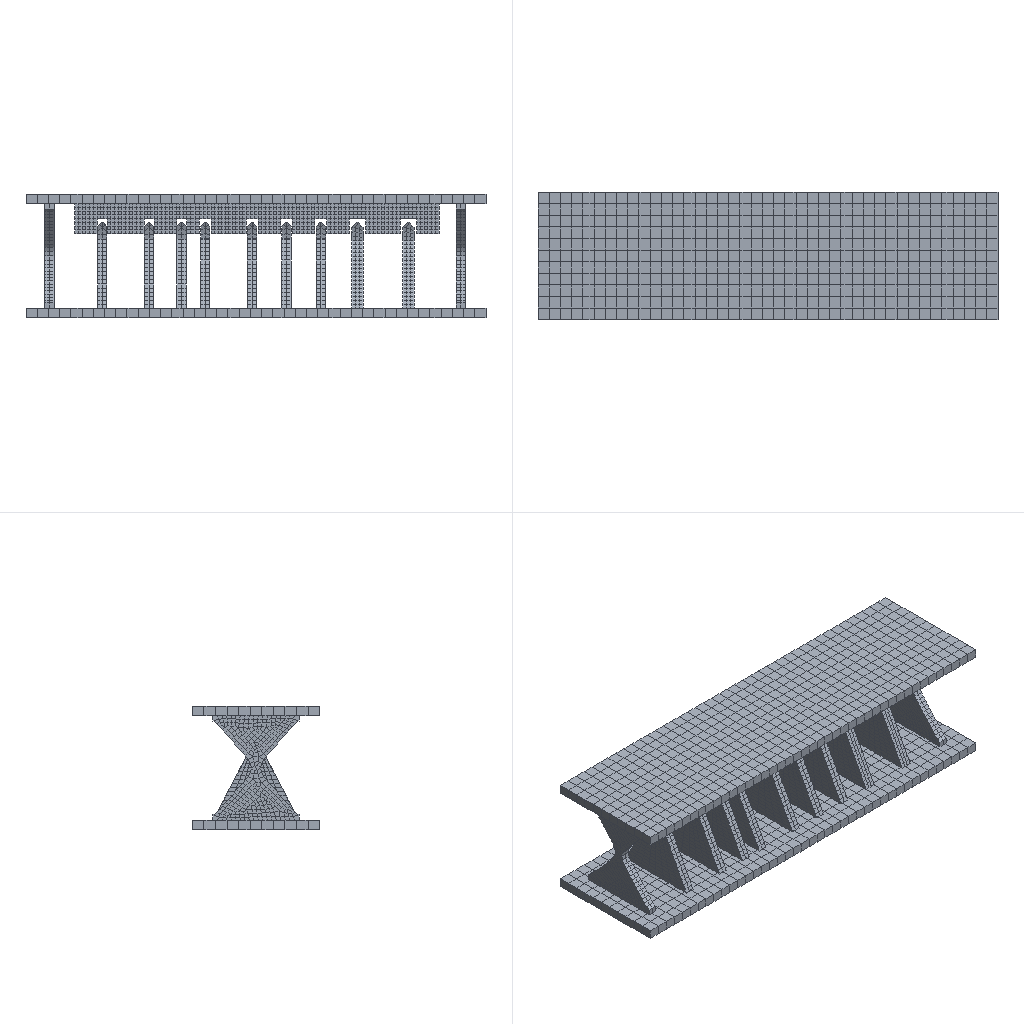Simulation study | abaqus
Abaqus input file, long lists of numbers shortened:
*Heading
** Job name: deck-1 Model name: 0814
** Generated by: Abaqus/CAE 2024
*Preprint, echo=NO, model=NO, history=NO, contact=NO
**
** PARTS
**
*Part, name=Part-1
*Node
      1,      1227.62,         340.,          25.
      2,      1227.62,   309.091,          25.
** (1006 more lines like these left out)
*Element, type=C3D8R
  1,   25,   26,   38,   37,    1,    2,   14,   13
  2,   26,   27,   39,   38,    2,    3,   15,   14
** (449 more lines like these left out)
*Nset, nset=_PickedSet5, internal, generate
    1,  1008,     1
*Elset, elset=_PickedSet5, internal, generate
   1,  451,    1
** Section: q235
*Solid Section, elset=_PickedSet5, controls=EC-1, material=q235
,
*End Part
**
*Part, name=Part-7
*Node
      1,   51318.848,   20056.129,           0.
      2,      51308.5,   20050.193,           0.
** (1084 more lines like these left out)
*Element, type=C3D8R
  1,  119,    1,    2,  145,  481,  363,  364,  507
  2,    1,  119,  116,   23,  363,  481,  478,  385
** (622 more lines like these left out)
*Nset, nset=Set-1, generate
    1,  1086,     1
*Elset, elset=Set-1, generate
   1,  624,    1
** Section: Section-2
*Solid Section, elset=Set-1, material=q235
,
*End Part
**
*Part, name=Part-8
*Node
      1,   44.972,         218.,           0.
      2,   50.449,         230.,          10.
** (601 more lines like these left out)
*Element, type=C3D8R
 1, 164,  20, 157, 481,  18,   1,  19, 155
 2, 165,  21, 158, 480, 164,  20, 157, 481
** (334 more lines like these left out)
*Nset, nset=Set-1, generate
   1,  603,    1
*Elset, elset=Set-1, generate
   1,  336,    1
** Section: Section-2
*Solid Section, elset=Set-1, material=q235
,
*End Part
**
*Part, name=Part-9
*Node
      1,  -916.483,   84.154,           0.
      2,  -916.483,   84.154,          40.
** (4008 more lines like these left out)
*Element, type=C3D8R
 1,  158, 1029, 2787,  999,    1,  121,  969,  136
 2, 1029, 1030, 2788, 2787,  121,  122,  970,  969
** (2638 more lines like these left out)
*Nset, nset=Set-1, generate
    1,  4010,     1
*Elset, elset=Set-1, generate
    1,  2640,     1
** Section: Section-2
*Solid Section, elset=Set-1, material=q235
,
*End Part
**
*Part, name=Part-10
*Node
      1,   4.129,   256.243,          25.
      2,   4.785,   252.357,          25.
** (558 more lines like these left out)
*Element, type=C3D8R
 1,  36,  43, 171, 165,   1,   2,  21,  22
 2, 165, 171,  42,  25,  22,  21,   3,   4
** (306 more lines like these left out)
*Nset, nset=Set-1
   1,   2,   3,   4,   5,   6,   7,   8,  17,  18,  19,  20,  21,  22,  23,  24
  25,  26,  27,  28,  29,  30,  31,  32,  33,  34,  35,  36,  37,  38,  39,  40
** (27 more lines like these left out)
*Elset, elset=Set-1
   1,   2,   3,   4,   5,   6,   7,   8,   9,  10,  11,  12,  13,  14,  71,  72
  73,  74,  75,  76,  77,  78,  79,  80,  81,  82,  83,  84,  85,  86,  87,  88
** (14 more lines like these left out)
*Nset, nset=_PickedSet10, internal, generate
   1,  560,    1
*Elset, elset=_PickedSet10, internal, generate
   1,  308,    1
** Section: Section-2
*Solid Section, elset=_PickedSet10, material=q235
,
*End Part
**
*Part, name=Part-11
*Node
      1,  -175.665,   409.503,         17.5
      2,  -105.665,   409.503,         17.5
** (878 more lines like these left out)
*Element, type=C3D8R
  1,   4,  22,   7,   1,  44,  62,  47,  41
  2,  22,  21,   8,   7,  62,  61,  48,  47
** (565 more lines like these left out)
*Nset, nset=Set-1, generate
   1,  880,    1
*Elset, elset=Set-1, generate
   1,  567,    1
** Section: Section-2
*Solid Section, elset=Set-1, material=q235
,
*End Part
**
**
** ASSEMBLY
**
*Assembly, name=Assembly
**
*Instance, name=Part-1-1, part=Part-1
*End Instance
**
*Instance, name=Part-1-1-lin-2-1, part=Part-1
          0.,           0.,         305.
*End Instance
**
*Instance, name=Part-7-1, part=Part-7
50.,     -51253.5, -20010.046
50.,     -51253.5, -20010.046, 50.577, -51252.923, -20009.469,         120.
*End Instance
**
*Instance, name=Part-7-1-lin-2-1, part=Part-7
     1147.62,     -51253.5, -20010.046
     1147.62,     -51253.5, -20010.046, 1148.197, -51252.923, -20009.469,         120.
*End Instance
**
*Instance, name=Part-9-1, part=Part-9
 1106.483,         190.,   180.846
 1106.483,         190.,   180.846, 1107.483,         190.,   180.846, 90.
*End Instance
**
*Instance, name=Part-8-1, part=Part-8
      190.85,   152.051,          25.
      190.85,   152.051,          25., 191.427, 152.628, 25.577,         120.
*End Instance
**
*Instance, name=Part-8-1-lin-1-2, part=Part-8
      315.85,   152.051,          25.
      315.85,   152.051,          25., 316.427, 152.628, 25.577,         120.
*End Instance
**
*Instance, name=Part-8-1-lin-1-2-lin-2-1, part=Part-8
      402.55,   152.051,          25.
      402.55,   152.051,          25., 403.127, 152.628, 25.577,         120.
*End Instance
**
*Instance, name=Part-10-1, part=Part-10
      465.85,   184.157,    -44.124
      465.85,   184.157,    -44.124, 466.427, 184.734, -43.547,         120.
*End Instance
**
*Instance, name=Part-10-1-lin-2-1, part=Part-10
      590.85,   184.157,    -44.124
      590.85,   184.157,    -44.124, 591.427, 184.734, -43.547,         120.
*End Instance
**
*Instance, name=Part-10-1-lin-3-1, part=Part-10
      774.37,   184.157,    -44.124
      774.37,   184.157,    -44.124, 774.947, 184.734, -43.547,         120.
*End Instance
**
*Instance, name=Part-10-1-lin-4-1, part=Part-10
      682.61,   184.157,    -44.124
      682.61,   184.157,    -44.124, 683.187, 184.734, -43.547,         120.
*End Instance
**
*Instance, name=Part-11-1, part=Part-11
      869.52,   310.665,   -154.503
      869.52,   310.665,   -154.503, 870.097, 311.242, -153.925,         120.
*End Instance
**
*Instance, name=Part-11-1-lin-2-1, part=Part-11
     1005.85,   310.665,   -154.503
     1005.85,   310.665,   -154.503, 1006.427, 311.242, -153.925,         120.
*End Instance
**
*Node
      1,   613.81,         170.,         500.
*Node
      2,   613.81,         170.,        -200.
*Nset, nset=Set-1, instance=Part-1-1
   13,   14,   15,   16,   17,   18,   19,   20,   21,   22,   23,   24,   37,   38,   39,   40
   41,   42,   43,   44,   45,   46,   47,   48,   61,   62,   63,   64,   65,   66,   67,   68
** (30 more lines like these left out)
*Elset, elset=Set-1, instance=Part-1-1, generate
   1,  451,    1
*Nset, nset=Set-6
 2,
*Nset, nset=Set-7
 1,
*Nset, nset=m_Set-5
 2,
*Nset, nset=rp1
 1,
*Nset, nset=rp2
 2,
*Nset, nset=_PickedSet71, internal
 1,
*Nset, nset=_PickedSet120, internal
 1,
*Nset, nset=_PickedSet121, internal
 2,
*Elset, elset=_m_Surf-12_S5, internal, instance=Part-1-1-lin-2-1, generate
   1,  451,    1
*Surface, type=ELEMENT, name=m_Surf-12
_m_Surf-12_S5, S5
*Elset, elset=_m_Surf-13_S3, internal, instance=Part-1-1, generate
   1,  451,    1
*Surface, type=ELEMENT, name=m_Surf-13
_m_Surf-13_S3, S3
*Elset, elset=_m_Surf-17_S3, internal, instance=Part-1-1, generate
   1,  451,    1
*Surface, type=ELEMENT, name=m_Surf-17
_m_Surf-17_S3, S3
*Elset, elset=_m_Surf-19_S5, internal, instance=Part-1-1-lin-2-1, generate
   1,  451,    1
*Surface, type=ELEMENT, name=m_Surf-19
_m_Surf-19_S5, S5
*Elset, elset=_m_Surf-28_S5, internal, instance=Part-8-1
  82,  83,  84,  85,  86,  87,  88,  89,  90,  91,  92,  93,  94,  95,  96,  97
  98, 116, 117, 118, 119, 120, 121, 122, 123, 124, 125, 126, 127, 128, 129, 130
** (7 more lines like these left out)
*Elset, elset=_m_Surf-28_S5, internal, instance=Part-8-1-lin-1-2
  82,  83,  84,  85,  86,  87,  88,  89,  90,  91,  92,  93,  94,  95,  96,  97
  98, 116, 117, 118, 119, 120, 121, 122, 123, 124, 125, 126, 127, 128, 129, 130
** (7 more lines like these left out)
*Elset, elset=_m_Surf-28_S5, internal, instance=Part-8-1-lin-1-2-lin-2-1
  82,  83,  84,  85,  86,  87,  88,  89,  90,  91,  92,  93,  94,  95,  96,  97
  98, 116, 117, 118, 119, 120, 121, 122, 123, 124, 125, 126, 127, 128, 129, 130
** (7 more lines like these left out)
*Elset, elset=_m_Surf-28_S5, internal, instance=Part-10-1-lin-2-1, generate
  2,  14,   2
*Elset, elset=_m_Surf-28_S5, internal, instance=Part-10-1-lin-4-1, generate
  2,  14,   2
*Elset, elset=_m_Surf-28_S5, internal, instance=Part-10-1, generate
  2,  14,   2
*Elset, elset=_m_Surf-28_S5, internal, instance=Part-10-1-lin-3-1, generate
  2,  14,   2
*Elset, elset=_m_Surf-28_S3, internal, instance=Part-8-1
  65,  66,  67,  68,  69,  70,  71,  72,  73,  74,  75,  76,  77,  78,  79,  80
  81,  99, 100, 101, 102, 103, 104, 105, 106, 107, 108, 109, 110, 111, 112, 113
** (7 more lines like these left out)
*Elset, elset=_m_Surf-28_S3, internal, instance=Part-8-1-lin-1-2
  65,  66,  67,  68,  69,  70,  71,  72,  73,  74,  75,  76,  77,  78,  79,  80
  81,  99, 100, 101, 102, 103, 104, 105, 106, 107, 108, 109, 110, 111, 112, 113
** (7 more lines like these left out)
*Elset, elset=_m_Surf-28_S3, internal, instance=Part-8-1-lin-1-2-lin-2-1
  65,  66,  67,  68,  69,  70,  71,  72,  73,  74,  75,  76,  77,  78,  79,  80
  81,  99, 100, 101, 102, 103, 104, 105, 106, 107, 108, 109, 110, 111, 112, 113
** (7 more lines like these left out)
*Elset, elset=_m_Surf-28_S3, internal, instance=Part-10-1-lin-2-1, generate
  1,  13,   2
*Elset, elset=_m_Surf-28_S3, internal, instance=Part-10-1-lin-4-1, generate
  1,  13,   2
*Elset, elset=_m_Surf-28_S3, internal, instance=Part-10-1, generate
  1,  13,   2
*Elset, elset=_m_Surf-28_S3, internal, instance=Part-10-1-lin-3-1, generate
  1,  13,   2
*Elset, elset=_m_Surf-28_S4, internal, instance=Part-10-1-lin-2-1, generate
  72,  308,    2
*Elset, elset=_m_Surf-28_S4, internal, instance=Part-10-1-lin-4-1, generate
  72,  308,    2
*Elset, elset=_m_Surf-28_S4, internal, instance=Part-10-1, generate
  72,  308,    2
*Elset, elset=_m_Surf-28_S4, internal, instance=Part-10-1-lin-3-1, generate
  72,  308,    2
*Elset, elset=_m_Surf-28_S6, internal, instance=Part-10-1-lin-2-1, generate
  71,  307,    2
*Elset, elset=_m_Surf-28_S6, internal, instance=Part-10-1-lin-4-1, generate
  71,  307,    2
*Elset, elset=_m_Surf-28_S6, internal, instance=Part-10-1, generate
  71,  307,    2
*Elset, elset=_m_Surf-28_S6, internal, instance=Part-10-1-lin-3-1, generate
  71,  307,    2
*Elset, elset=_m_Surf-28_S1, internal, instance=Part-10-1-lin-2-1
 13, 14
*Elset, elset=_m_Surf-28_S1, internal, instance=Part-10-1-lin-4-1
 13, 14
*Elset, elset=_m_Surf-28_S1, internal, instance=Part-10-1
 13, 14
*Elset, elset=_m_Surf-28_S1, internal, instance=Part-10-1-lin-3-1
 13, 14
*Elset, elset=_m_Surf-28_S2, internal, instance=Part-10-1-lin-2-1
 1, 2
*Elset, elset=_m_Surf-28_S2, internal, instance=Part-10-1-lin-4-1
 1, 2
*Elset, elset=_m_Surf-28_S2, internal, instance=Part-10-1
 1, 2
*Elset, elset=_m_Surf-28_S2, internal, instance=Part-10-1-lin-3-1
 1, 2
*Surface, type=ELEMENT, name=m_Surf-28
_m_Surf-28_S5, S5
_m_Surf-28_S3, S3
_m_Surf-28_S4, S4
_m_Surf-28_S6, S6
_m_Surf-28_S2, S2
_m_Surf-28_S1, S1
*Elset, elset=_m_Surf-30_S4, internal, instance=Part-8-1
  1,  2,  3,  4,  5,  6,  7,  8,  9, 10, 11, 12, 13, 14, 15, 16
 25, 26, 27, 28, 29, 30, 31, 32, 36, 37, 38, 39, 40, 44, 48, 52
** (1 more lines like these left out)
*Elset, elset=_m_Surf-30_S4, internal, instance=Part-8-1-lin-1-2
  1,  2,  3,  4,  5,  6,  7,  8,  9, 10, 11, 12, 13, 14, 15, 16
 25, 26, 27, 28, 29, 30, 31, 32, 36, 37, 38, 39, 40, 44, 48, 52
** (1 more lines like these left out)
*Elset, elset=_m_Surf-30_S4, internal, instance=Part-8-1-lin-1-2-lin-2-1
  1,  2,  3,  4,  5,  6,  7,  8,  9, 10, 11, 12, 13, 14, 15, 16
 25, 26, 27, 28, 29, 30, 31, 32, 36, 37, 38, 39, 40, 44, 48, 52
** (1 more lines like these left out)
*Elset, elset=_m_Surf-30_S4, internal, instance=Part-10-1-lin-2-1
  15,  16,  17,  18,  19,  20,  21,  22,  23,  24,  25,  26,  33,  34,  35,  36
  37,  38,  42,  43,  44,  45,  46,  50,  54,  58,  62,  66,  70,  72,  74,  76
** (8 more lines like these left out)
*Elset, elset=_m_Surf-30_S4, internal, instance=Part-10-1-lin-4-1
  15,  16,  17,  18,  19,  20,  21,  22,  23,  24,  25,  26,  33,  34,  35,  36
  37,  38,  42,  43,  44,  45,  46,  50,  54,  58,  62,  66,  70,  72,  74,  76
** (8 more lines like these left out)
*Elset, elset=_m_Surf-30_S4, internal, instance=Part-11-1-lin-2-1, generate
   9,  549,   27
*Elset, elset=_m_Surf-30_S4, internal, instance=Part-10-1
  15,  16,  17,  18,  19,  20,  21,  22,  23,  24,  25,  26,  33,  34,  35,  36
  37,  38,  42,  43,  44,  45,  46,  50,  54,  58,  62,  66,  70,  72,  74,  76
** (8 more lines like these left out)
*Elset, elset=_m_Surf-30_S4, internal, instance=Part-11-1, generate
   9,  549,   27
*Elset, elset=_m_Surf-30_S4, internal, instance=Part-10-1-lin-3-1
  15,  16,  17,  18,  19,  20,  21,  22,  23,  24,  25,  26,  33,  34,  35,  36
  37,  38,  42,  43,  44,  45,  46,  50,  54,  58,  62,  66,  70,  72,  74,  76
** (8 more lines like these left out)
*Elset, elset=_m_Surf-30_S3, internal, instance=Part-8-1
   1,   2,   3,   4,   5,   6,   7,   8,   9,  10,  11,  12,  13,  14,  15,  16
  17,  18,  19,  20,  21,  22,  23,  24,  33,  34,  35,  36,  37,  49,  50,  51
** (10 more lines like these left out)
*Elset, elset=_m_Surf-30_S3, internal, instance=Part-8-1-lin-1-2
   1,   2,   3,   4,   5,   6,   7,   8,   9,  10,  11,  12,  13,  14,  15,  16
  17,  18,  19,  20,  21,  22,  23,  24,  33,  34,  35,  36,  37,  49,  50,  51
** (10 more lines like these left out)
*Elset, elset=_m_Surf-30_S3, internal, instance=Part-8-1-lin-1-2-lin-2-1
   1,   2,   3,   4,   5,   6,   7,   8,   9,  10,  11,  12,  13,  14,  15,  16
  17,  18,  19,  20,  21,  22,  23,  24,  33,  34,  35,  36,  37,  49,  50,  51
** (10 more lines like these left out)
*Elset, elset=_m_Surf-30_S3, internal, instance=Part-10-1-lin-2-1
   1,   3,   5,   7,   9,  11,  13,  15,  16,  17,  18,  19,  20,  21,  22,  23
  24,  25,  26,  27,  28,  29,  30,  31,  32,  39,  40,  41,  42,  43,  55,  56
** (3 more lines like these left out)
*Elset, elset=_m_Surf-30_S3, internal, instance=Part-10-1-lin-4-1
   1,   3,   5,   7,   9,  11,  13,  15,  16,  17,  18,  19,  20,  21,  22,  23
  24,  25,  26,  27,  28,  29,  30,  31,  32,  39,  40,  41,  42,  43,  55,  56
** (3 more lines like these left out)
*Elset, elset=_m_Surf-30_S3, internal, instance=Part-11-1-lin-2-1
   1,   2,   3,   4,   5,   6,   7,   8,   9,  26,  27,  28,  29,  30,  31,  32
  33,  34,  35,  36,  53,  54,  55,  56,  57,  58,  59,  60,  61,  62,  63,  80
** (13 more lines like these left out)
*Elset, elset=_m_Surf-30_S3, internal, instance=Part-10-1
   1,   3,   5,   7,   9,  11,  13,  15,  16,  17,  18,  19,  20,  21,  22,  23
  24,  25,  26,  27,  28,  29,  30,  31,  32,  39,  40,  41,  42,  43,  55,  56
** (3 more lines like these left out)
*Elset, elset=_m_Surf-30_S3, internal, instance=Part-11-1
   1,   2,   3,   4,   5,   6,   7,   8,   9,  26,  27,  28,  29,  30,  31,  32
  33,  34,  35,  36,  53,  54,  55,  56,  57,  58,  59,  60,  61,  62,  63,  80
** (13 more lines like these left out)
*Elset, elset=_m_Surf-30_S3, internal, instance=Part-10-1-lin-3-1
   1,   3,   5,   7,   9,  11,  13,  15,  16,  17,  18,  19,  20,  21,  22,  23
  24,  25,  26,  27,  28,  29,  30,  31,  32,  39,  40,  41,  42,  43,  55,  56
** (3 more lines like these left out)
*Elset, elset=_m_Surf-30_S2, internal, instance=Part-8-1
  1,  5,  9, 13, 17, 18, 25, 26, 33, 34, 35, 36, 37, 38, 39, 40
 41, 42, 43, 44, 45, 46, 47, 48, 57, 61, 65, 66, 67, 68, 69, 70
** (2 more lines like these left out)
*Elset, elset=_m_Surf-30_S2, internal, instance=Part-8-1-lin-1-2
  1,  5,  9, 13, 17, 18, 25, 26, 33, 34, 35, 36, 37, 38, 39, 40
 41, 42, 43, 44, 45, 46, 47, 48, 57, 61, 65, 66, 67, 68, 69, 70
** (2 more lines like these left out)
*Elset, elset=_m_Surf-30_S2, internal, instance=Part-8-1-lin-1-2-lin-2-1
  1,  5,  9, 13, 17, 18, 25, 26, 33, 34, 35, 36, 37, 38, 39, 40
 41, 42, 43, 44, 45, 46, 47, 48, 57, 61, 65, 66, 67, 68, 69, 70
** (2 more lines like these left out)
*Elset, elset=_m_Surf-30_S2, internal, instance=Part-10-1-lin-2-1
  1,  2, 15, 18, 21, 24, 27, 28, 33, 34, 39, 40, 41, 42, 43, 44
 45, 46, 47, 48, 49, 50, 51, 52, 53, 54, 63, 64, 65, 66, 67, 68
** (1 more lines like these left out)
*Elset, elset=_m_Surf-30_S2, internal, instance=Part-10-1-lin-4-1
  1,  2, 15, 18, 21, 24, 27, 28, 33, 34, 39, 40, 41, 42, 43, 44
 45, 46, 47, 48, 49, 50, 51, 52, 53, 54, 63, 64, 65, 66, 67, 68
** (1 more lines like these left out)
*Elset, elset=_m_Surf-30_S2, internal, instance=Part-10-1
  1,  2, 15, 18, 21, 24, 27, 28, 33, 34, 39, 40, 41, 42, 43, 44
 45, 46, 47, 48, 49, 50, 51, 52, 53, 54, 63, 64, 65, 66, 67, 68
** (1 more lines like these left out)
*Elset, elset=_m_Surf-30_S2, internal, instance=Part-10-1-lin-3-1
  1,  2, 15, 18, 21, 24, 27, 28, 33, 34, 39, 40, 41, 42, 43, 44
 45, 46, 47, 48, 49, 50, 51, 52, 53, 54, 63, 64, 65, 66, 67, 68
** (1 more lines like these left out)
*Elset, elset=_m_Surf-30_S5, internal, instance=Part-8-1
  82,  83,  84,  85,  86,  87,  88,  89,  90,  91,  92,  93,  94,  95,  96,  97
  98, 116, 117, 118, 119, 120, 121, 122, 123, 124, 125, 126, 127, 128, 129, 130
** (7 more lines like these left out)
*Elset, elset=_m_Surf-30_S5, internal, instance=Part-8-1-lin-1-2
  82,  83,  84,  85,  86,  87,  88,  89,  90,  91,  92,  93,  94,  95,  96,  97
  98, 116, 117, 118, 119, 120, 121, 122, 123, 124, 125, 126, 127, 128, 129, 130
** (7 more lines like these left out)
*Elset, elset=_m_Surf-30_S5, internal, instance=Part-8-1-lin-1-2-lin-2-1
  82,  83,  84,  85,  86,  87,  88,  89,  90,  91,  92,  93,  94,  95,  96,  97
  98, 116, 117, 118, 119, 120, 121, 122, 123, 124, 125, 126, 127, 128, 129, 130
** (7 more lines like these left out)
*Elset, elset=_m_Surf-30_S5, internal, instance=Part-10-1-lin-2-1
   2,   4,   6,   8,  10,  12,  14,  83,  84,  97,  98, 111, 112, 125, 126, 139
 140, 153, 154, 167, 168, 181, 182, 195, 196, 209, 210, 223, 224, 237, 238, 251
** (1 more lines like these left out)
*Elset, elset=_m_Surf-30_S5, internal, instance=Part-10-1-lin-4-1
   2,   4,   6,   8,  10,  12,  14,  83,  84,  97,  98, 111, 112, 125, 126, 139
 140, 153, 154, 167, 168, 181, 182, 195, 196, 209, 210, 223, 224, 237, 238, 251
** (1 more lines like these left out)
*Elset, elset=_m_Surf-30_S5, internal, instance=Part-11-1-lin-2-1
  10,  11,  37,  38,  64,  65,  91,  92, 118, 119, 145, 146, 172, 173, 199, 200
 226, 227, 253, 254, 280, 281, 307, 308, 334, 335, 361, 362, 388, 389, 415, 416
** (1 more lines like these left out)
*Elset, elset=_m_Surf-30_S5, internal, instance=Part-10-1
   2,   4,   6,   8,  10,  12,  14,  83,  84,  97,  98, 111, 112, 125, 126, 139
 140, 153, 154, 167, 168, 181, 182, 195, 196, 209, 210, 223, 224, 237, 238, 251
** (1 more lines like these left out)
*Elset, elset=_m_Surf-30_S5, internal, instance=Part-11-1
  10,  11,  37,  38,  64,  65,  91,  92, 118, 119, 145, 146, 172, 173, 199, 200
 226, 227, 253, 254, 280, 281, 307, 308, 334, 335, 361, 362, 388, 389, 415, 416
** (1 more lines like these left out)
*Elset, elset=_m_Surf-30_S5, internal, instance=Part-10-1-lin-3-1
   2,   4,   6,   8,  10,  12,  14,  83,  84,  97,  98, 111, 112, 125, 126, 139
 140, 153, 154, 167, 168, 181, 182, 195, 196, 209, 210, 223, 224, 237, 238, 251
** (1 more lines like these left out)
*Elset, elset=_m_Surf-30_S1, internal, instance=Part-8-1, generate
 303,  336,    1
*Elset, elset=_m_Surf-30_S1, internal, instance=Part-8-1-lin-1-2, generate
 303,  336,    1
*Elset, elset=_m_Surf-30_S1, internal, instance=Part-8-1-lin-1-2-lin-2-1, generate
 303,  336,    1
*Elset, elset=_m_Surf-30_S1, internal, instance=Part-10-1-lin-2-1
 13, 14
*Elset, elset=_m_Surf-30_S1, internal, instance=Part-10-1-lin-4-1
 13, 14
*Elset, elset=_m_Surf-30_S1, internal, instance=Part-11-1-lin-2-1, generate
  1,  27,   1
*Elset, elset=_m_Surf-30_S1, internal, instance=Part-10-1
 13, 14
*Elset, elset=_m_Surf-30_S1, internal, instance=Part-11-1, generate
  1,  27,   1
*Elset, elset=_m_Surf-30_S1, internal, instance=Part-10-1-lin-3-1
 13, 14
*Elset, elset=_m_Surf-30_S6, internal, instance=Part-10-1-lin-2-1, generate
  71,  307,    2
*Elset, elset=_m_Surf-30_S6, internal, instance=Part-10-1-lin-4-1, generate
  71,  307,    2
*Elset, elset=_m_Surf-30_S6, internal, instance=Part-11-1-lin-2-1
   1,  10,  12,  14,  16,  18,  20,  22,  24,  26,  28,  37,  39,  41,  43,  45
  47,  49,  51,  53,  55,  64,  66,  68,  70,  72,  74,  76,  78,  80,  82,  91
** (12 more lines like these left out)
*Elset, elset=_m_Surf-30_S6, internal, instance=Part-10-1, generate
  71,  307,    2
*Elset, elset=_m_Surf-30_S6, internal, instance=Part-11-1
   1,  10,  12,  14,  16,  18,  20,  22,  24,  26,  28,  37,  39,  41,  43,  45
  47,  49,  51,  53,  55,  64,  66,  68,  70,  72,  74,  76,  78,  80,  82,  91
** (12 more lines like these left out)
*Elset, elset=_m_Surf-30_S6, internal, instance=Part-10-1-lin-3-1, generate
  71,  307,    2
*Surface, type=ELEMENT, name=m_Surf-30
_m_Surf-30_S4, S4
_m_Surf-30_S3, S3
_m_Surf-30_S2, S2
_m_Surf-30_S6, S6
_m_Surf-30_S5, S5
_m_Surf-30_S1, S1
*Elset, elset=_s_Surf-1_S3, internal, instance=Part-1-1, generate
   1,  451,    1
*Surface, type=ELEMENT, name=s_Surf-1
_s_Surf-1_S3, S3
*Elset, elset=_s_Surf-3_S5, internal, instance=Part-1-1-lin-2-1, generate
   1,  451,    1
*Surface, type=ELEMENT, name=s_Surf-3
_s_Surf-3_S5, S5
*Elset, elset=_s_Surf-14_S4, internal, instance=Part-1-1, generate
  11,  451,   11
*Surface, type=ELEMENT, name=s_Surf-14
_s_Surf-14_S4, S4
*Elset, elset=_s_Surf-17_S5, internal, instance=Part-1-1, generate
   1,  451,    1
*Surface, type=ELEMENT, name=s_Surf-17
_s_Surf-17_S5, S5
*Elset, elset=_s_Surf-26_S4, internal, instance=Part-7-1
  15, 327
*Elset, elset=_s_Surf-26_S4, internal, instance=Part-7-1-lin-2-1
  15, 327
*Elset, elset=_s_Surf-26_S4, internal, instance=Part-9-1
 2036, 2040, 2044, 2048, 2052, 2056, 2060, 2064, 2068, 2072, 2076, 2080, 2132, 2136, 2140, 2144
 2148, 2152, 2156, 2160, 2164, 2168, 2172, 2176, 2372, 2376, 2380, 2384, 2388, 2392, 2396, 2400
** (1 more lines like these left out)
*Elset, elset=_s_Surf-26_S5, internal, instance=Part-7-1
  16,  33,  42, 111, 124, 133, 135, 138, 328, 345, 354, 423, 436, 445, 447, 450
*Elset, elset=_s_Surf-26_S5, internal, instance=Part-7-1-lin-2-1
  16,  33,  42, 111, 124, 133, 135, 138, 328, 345, 354, 423, 436, 445, 447, 450
*Elset, elset=_s_Surf-26_S3, internal, instance=Part-7-1
  35,  37,  39,  48, 114, 115, 116, 118, 119, 143, 347, 349, 351, 360, 426, 427
 428, 430, 431, 455
*Elset, elset=_s_Surf-26_S3, internal, instance=Part-7-1-lin-2-1
  35,  37,  39,  48, 114, 115, 116, 118, 119, 143, 347, 349, 351, 360, 426, 427
 428, 430, 431, 455
*Elset, elset=_s_Surf-26_S1, internal, instance=Part-9-1
   73,   74,   75,   76,   77,   78,   79,   80,   81,   82,   83,   84,   85,   86,   87,   88
   89,   90,   91,   92,   93,   94,   95,   96,  217,  218,  219,  220,  221,  222,  223,  224
** (18 more lines like these left out)
*Elset, elset=_s_Surf-26_S2, internal, instance=Part-9-1, generate
 2497,  2532,     1
*Surface, type=ELEMENT, name=s_Surf-26
_s_Surf-26_S4, S4
_s_Surf-26_S5, S5
_s_Surf-26_S2, S2
_s_Surf-26_S3, S3
_s_Surf-26_S1, S1
*Elset, elset=_s_Surf-27_S5, internal, instance=Part-7-1
  20,  22,  62,  79,  87,  90,  95,  97, 154, 332, 334, 374, 391, 399, 402, 407
 409, 466
*Elset, elset=_s_Surf-27_S5, internal, instance=Part-7-1-lin-2-1
  20,  22,  62,  79,  87,  90,  95,  97, 154, 332, 334, 374, 391, 399, 402, 407
 409, 466
*Elset, elset=_s_Surf-27_S3, internal, instance=Part-7-1
  69,  76,  77,  81,  85,  86,  89,  98, 106, 381, 388, 389, 393, 397, 398, 401
 410, 418
*Elset, elset=_s_Surf-27_S3, internal, instance=Part-7-1-lin-2-1
  69,  76,  77,  81,  85,  86,  89,  98, 106, 381, 388, 389, 393, 397, 398, 401
 410, 418
*Elset, elset=_s_Surf-27_S6, internal, instance=Part-7-1
  72, 384
*Elset, elset=_s_Surf-27_S6, internal, instance=Part-7-1-lin-2-1
  72, 384
*Elset, elset=_s_Surf-27_S4, internal, instance=Part-8-1-lin-1-2, generate
  81,  336,   17
*Elset, elset=_s_Surf-27_S4, internal, instance=Part-8-1, generate
  81,  336,   17
*Elset, elset=_s_Surf-27_S4, internal, instance=Part-8-1-lin-1-2-lin-2-1, generate
  81,  336,   17
*Elset, elset=_s_Surf-27_S2, internal, instance=Part-10-1-lin-4-1, generate
 295,  308,    1
*Elset, elset=_s_Surf-27_S2, internal, instance=Part-10-1-lin-2-1, generate
 295,  308,    1
*Elset, elset=_s_Surf-27_S2, internal, instance=Part-11-1-lin-2-1, generate
 541,  567,    1
*Elset, elset=_s_Surf-27_S2, internal, instance=Part-10-1, generate
 295,  308,    1
*Elset, elset=_s_Surf-27_S2, internal, instance=Part-11-1, generate
 541,  567,    1
*Elset, elset=_s_Surf-27_S2, internal, instance=Part-10-1-lin-3-1, generate
 295,  308,    1
*Surface, type=ELEMENT, name=s_Surf-27
_s_Surf-27_S5, S5
_s_Surf-27_S3, S3
_s_Surf-27_S6, S6
_s_Surf-27_S4, S4
_s_Surf-27_S2, S2
*Elset, elset=_s_Surf-28_S5, internal, instance=Part-9-1
   21,   22,   23,   24,   45,   46,   47,   48,   69,   70,   71,   72,   93,   94,   95,   96
  869,  870,  871,  872,  893,  894,  895,  896,  917,  918,  919,  920,  941,  942,  943,  944
** (19 more lines like these left out)
*Elset, elset=_s_Surf-28_S4, internal, instance=Part-9-1
    4,    8,   12,   16,   20,   24,   28,   32,   36,   40,   44,   48,   52,   56,   60,   64
   68,   72,   76,   80,   84,   88,   92,   96,  100,  104,  108,  112,  116,  120,  124,  128
** (30 more lines like these left out)
*Elset, elset=_s_Surf-28_S6, internal, instance=Part-9-1
    1,    5,    9,   13,   17,   21,   25,   29,   33,   37,   41,   45,   49,   53,   57,   61
   65,   69,   73,   77,   81,   85,   89,   93,   97,  101,  105,  109,  113,  117,  121,  125
** (35 more lines like these left out)
*Elset, elset=_s_Surf-28_S3, internal, instance=Part-9-1
  945,  946,  947,  948,  969,  970,  971,  972,  993,  994,  995,  996, 1017, 1018, 1019, 1020
 1041, 1042, 1043, 1044, 1081, 1082, 1083, 1084, 1121, 1122, 1123, 1124, 1161, 1162, 1163, 1164
** (17 more lines like these left out)
*Elset, elset=_s_Surf-28_S2, internal, instance=Part-9-1
 1017, 1018, 1019, 1020, 1021, 1022, 1023, 1024, 1025, 1026, 1027, 1028, 1029, 1030, 1031, 1032
 1033, 1034, 1035, 1036, 1037, 1038, 1039, 1040, 1161, 1162, 1163, 1164, 1165, 1166, 1167, 1168
** (19 more lines like these left out)
*Elset, elset=_s_Surf-28_S1, internal, instance=Part-9-1, generate
 2017,  2032,     1
*Surface, type=ELEMENT, name=s_Surf-28
_s_Surf-28_S5, S5
_s_Surf-28_S4, S4
_s_Surf-28_S6, S6
_s_Surf-28_S2, S2
_s_Surf-28_S3, S3
_s_Surf-28_S1, S1
*Elset, elset=__PickedSurf70_S3, internal, instance=Part-1-1-lin-2-1, generate
   1,  451,    1
*Surface, type=ELEMENT, name=_PickedSurf70, internal
__PickedSurf70_S3, S3
** Constraint: Constraint-2
*Tie, name=Constraint-2, adjust=yes
s_Surf-26, m_Surf-12
** Constraint: Constraint-3
*Tie, name=Constraint-3, adjust=yes
s_Surf-27, m_Surf-13
** Constraint: Constraint-4
*Coupling, constraint name=Constraint-4, ref node=m_Set-5, surface=s_Surf-17
*Kinematic
** Constraint: rp-1
*Coupling, constraint name=rp-1, ref node=_PickedSet71, surface=_PickedSurf70
*Kinematic
*End Assembly
**
** ELEMENT CONTROLS
**
*Section Controls, name=EC-1, VISCOSITY=0.0001
1., 1., 1.
*Amplitude, name=Amp-1
             0.,              0.,              1.,              5.,              2.,              0.,              3.,             -5.
             4.,              0.,              5.,              5.,              6.,              0.,              7.,             -5.
             8.,              0.,              9.,              5.,             10.,              0.,             11.,             -5.
            12.,              0.,             13.,             10.,             14.,              0.,             15.,            -10.
            16.,              0.,             17.,             10.,             18.,              0.,             19.,            -10.
            20.,              0.,             21.,             10.,             22.,              0.,             23.,            -10.
            24.,              0.,             25.,             15.,             26.,              0.,             27.,            -15.
            28.,              0.,             29.,             15.,             30.,              0.,             31.,            -15.
            32.,              0.,             33.,             15.,             34.,              0.,             35.,            -15.
            36.,              0.,             37.,             20.,             38.,              0.,             39.,            -20.
            40.,              0.,             41.,             20.,             42.,              0.,             43.,            -20.
            44.,              0.,             45.,             20.,             46.,              0.,             47.,            -20.
            48.,              0.,             49.,             25.,             50.,              0.,             51.,            -25.
            52.,              0.,             53.,             25.,             54.,              0.,             55.,            -25.
            56.,              0.,             57.,             25.,             58.,              0.,             59.,            -25.
            60.,              0.,             61.,             30.,             62.,              0.,             63.,            -30.
            64.,              0.,             65.,             30.,             66.,              0.,             67.,            -30.
            68.,              0.,             69.,             30.,             70.,              0.,             71.,            -30.
            72.,              0.,             73.,             35.,             74.,              0.,             75.,            -35.
            76.,              0.,             77.,             35.,             78.,              0.,             79.,            -35.
            80.,              0.,             81.,             35.,             82.,              0.,             83.,            -35.
            84.,              0.,             85.,             40.,             86.,              0.,             87.,            -40.
            88.,              0.,             89.,             40.,             90.,              0.,             91.,            -40.
            92.,              0.,             93.,             40.,             94.,              0.,             95.,            -40.
            96.,              0.,             97.,             45.,             98.,              0.,             99.,            -45.
           100.,              0.,            101.,             45.,            102.,              0.,            103.,            -45.
           104.,              0.,            105.,             45.,            106.,              0.,            107.,            -45.
           108.,              0.,            109.,             50.,            110.,              0.,            111.,            -50.
           112.,              0.,            113.,             50.,            114.,              0.,            115.,            -50.
           116.,              0.,            117.,             50.,            118.,              0.,            119.,            -50.
           120.,              0.
*Amplitude, name=Amp-2
             0.,              0.,              1.,             0.5,              2.,              0.,              3.,            -0.5
             4.,              0.,              5.,            0.85,              6.,              0.,              7.,           -0.85
             8.,              0.,              9.,              2.,             10.,              0.,             11.,             -2.
            12.,              0.,             13.,            3.38,             14.,              0.,             15.,           -3.38
            16.,              0.,             17.,              5.,             18.,              0.,             19.,             -5.
            20.,              0.,             21.,            6.77,             22.,              0.,             23.,           -6.77
            24.,              0.,             25.,              8.,             26.,              0.,             27.,             -8.
            28.,              0.,             29.,           10.16,             30.,              0.,             31.,          -10.16
            32.,              0.,             33.,             15.,             34.,              0.,             35.,            -15.
            36.,              0.,             37.,             20.,             38.,              0.,             39.,            -20.
            40.,              0.,             41.,             25.,             42.,              0.,             43.,            -25.
            44.,              0.,             45.,             30.,             46.,              0.,             47.,            -30.
            48.,              0.,             49.,             35.,             50.,              0.,             51.,            -35.
            52.,              0.,             53.,             40.,             54.,              0.,             55.,            -40.
            56.,              0.,             57.,             45.,             58.,              0.,             59.,            -45.
            60.,              0.,             61.,             50.,             62.,              0.,             63.,            -50.
            64.,              0.
*Amplitude, name=Amp-3
             0.,              0.,              1.,             0.5,              2.,              0.,              3.,            -0.5
             4.,              0.,              5.,            0.85,              6.,              0.,              7.,           -0.85
             8.,              0.,              9.,              2.,             10.,              0.,             11.,             -2.
            12.,              0.,             13.,            3.38,             14.,              0.,             15.,           -3.38
            16.,              0.,             17.,              5.,             18.,              0.,             19.,             -5.
            20.,              0.,             21.,            6.77,             22.,              0.,             23.,           -6.77
            24.,              0.,             25.,              8.,             26.,              0.,             27.,             -8.
            28.,              0.,             29.,           10.16,             30.,              0.,             31.,          -10.16
            32.,              0.,             33.,             15.,             34.,              0.,             35.,            -15.
            36.,              0.,             37.,             20.,             38.,              0.,             39.,            -20.
            40.,              0.,             41.,             25.,             42.,              0.,             43.,            -25.
            44.,              0.,             45.,             30.,             46.,              0.,             47.,            -30.
            48.,              0.,             49.,             35.,             50.,              0.,             51.,            -35.
            52.,              0.,             53.,             40.,             54.,              0.,             55.,            -40.
            56.,              0.,             57.,             45.,             58.,              0.,             59.,            -45.
            60.,              0.,             61.,             50.,             62.,              0.,             63.,            -50.
            64.,              0.,             65.,             55.,             66.,              0.,             67.,            -55.
            68.,              0.,             69.,             60.,             70.,              0.,             71.,            -60.
            72.,              0.,             73.,             65.,             74.,              0.,             75.,            -65.
            76.,              0.,             77.,             70.,             78.,              0.,             79.,            -70.
            80.,              0.
**
** MATERIALS
**
*Material, name=q235
*Density
 7.85e-09,
*Elastic
206000., 0.3
*Plastic
220.,  0.
350., 0.2
**
** INTERACTION PROPERTIES
**
*Surface Interaction, name=IntProp-1
1.,
*Friction, slip tolerance=0.005
 0.3,
*Surface Behavior, pressure-overclosure=HARD
*Contact Damping, definition=DAMPING COEFFICIENT
0.1, 200., 0.
**
** BOUNDARY CONDITIONS
**
** Name: BC-4 Type: Symmetry/Antisymmetry/Encastre
*Boundary
_PickedSet121, ENCASTRE
**
** INTERACTIONS
**
** Interaction: Int-1
*Contact Pair, interaction=IntProp-1, type=SURFACE TO SURFACE
s_Surf-28, m_Surf-30
** ----------------------------------------------------------------
**
** STEP: Step-1
**
*Step, name=Step-1, nlgeom=YES, inc=1000000
*Static, stabilize=0.0002, allsdtol=0.05, continue=NO
0.1, 80., 6.4e-08, 0.5
**
** BOUNDARY CONDITIONS
**
** Name: BC-3 Type: Displacement/Rotation
*Boundary, amplitude=Amp-3
_PickedSet120, 1, 1, 1.
_PickedSet120, 2, 2
_PickedSet120, 3, 3
_PickedSet120, 4, 4
_PickedSet120, 5, 5
_PickedSet120, 6, 6
**
** CONTROLS
**
*Controls, reset
*Controls, analysis=discontinuous
*Controls, parameters=time incrementation
, , , , , , , 20, , ,
**
** OUTPUT REQUESTS
**
*Restart, write, frequency=0
**
** FIELD OUTPUT: F-Output-1
**
*Output, field
*Node Output
RF, U
*Element Output, directions=YES
LE, PE, PEEQ, PEMAG, S
**
** HISTORY OUTPUT: H-Output-1
**
*Output, history, variable=PRESELECT
*End Step